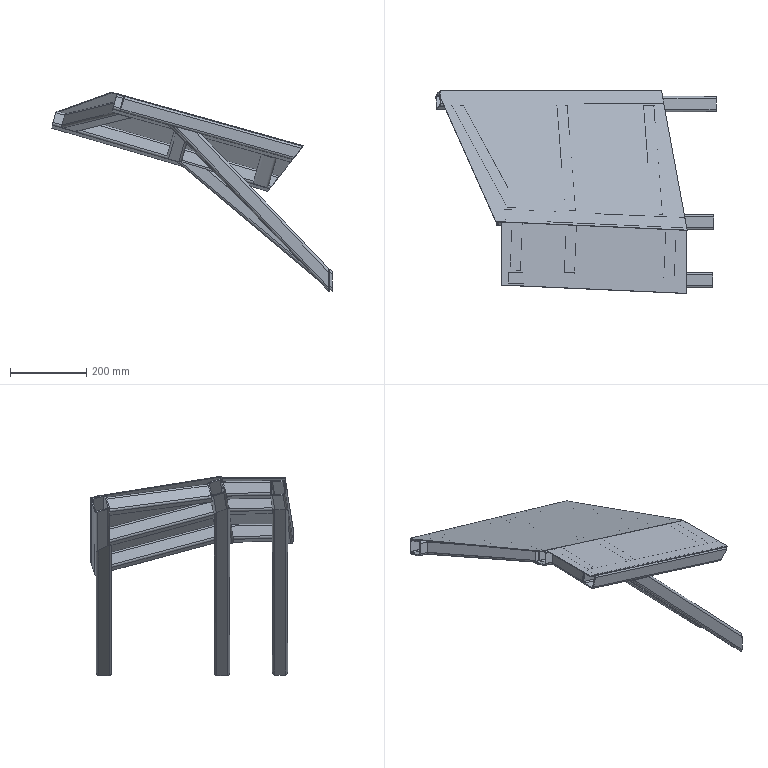Part | STEP file | left fixed inclined baffle (down) | 14 solids | 229 faces | box 733.286 x 530.621 x 522.776 mm | volume 2414380 mm3 | plane 133 | cylinder 96 | commonest cylinder face diameters 6 x48 12 x48